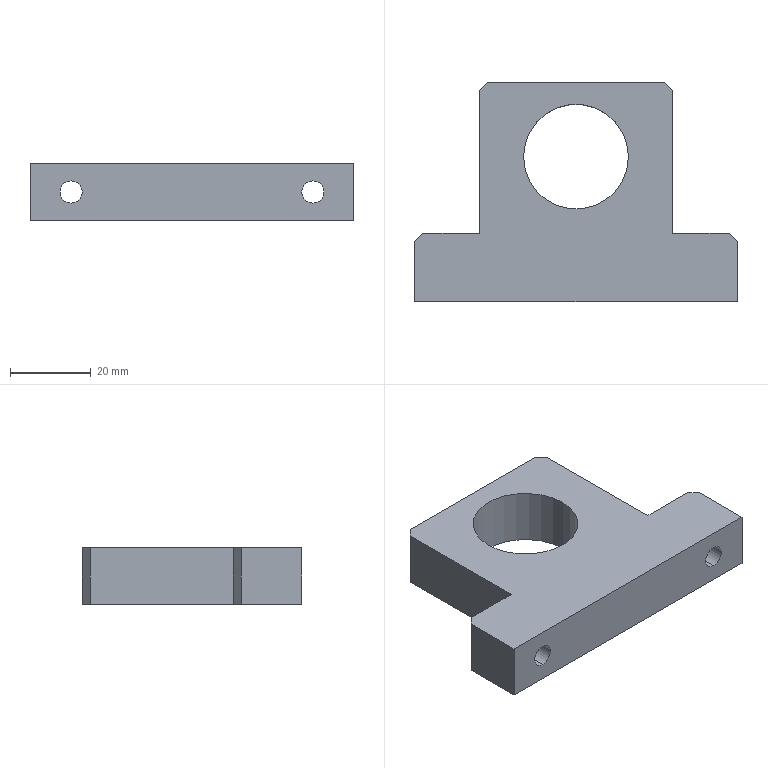Part | STEP file | lead screw support block - COMPANY_A version | 1 solid | 20 faces | box 80 x 54.5 x 14 mm | volume 35887 mm3 | plane 14 | cylinder 6 | commonest cylinder face diameters 5.5 x4 26 x2